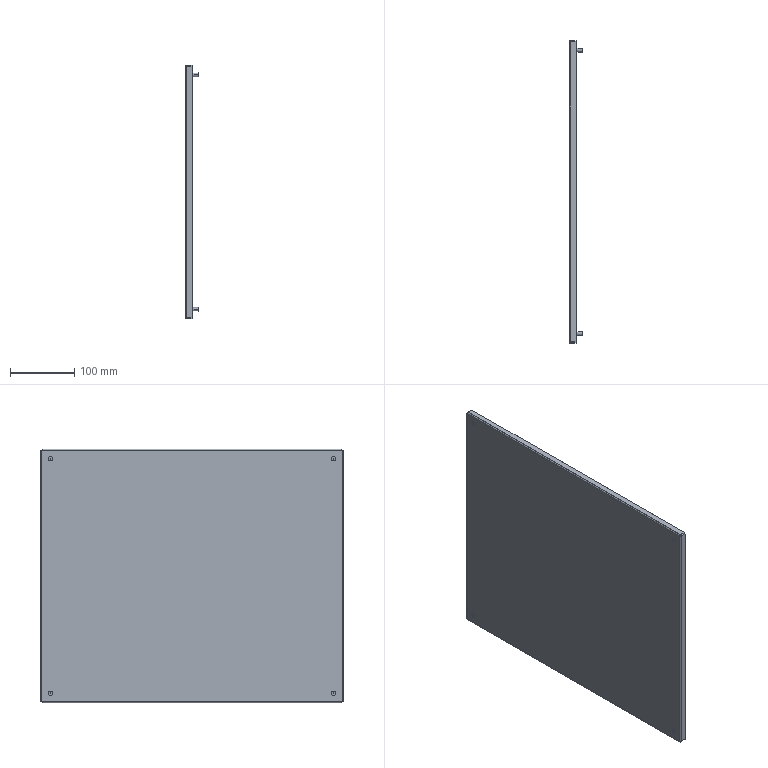Part | SolidWorks | features BaseBody 5 | 5 solids | 66 faces | box 20 x 472 x 396 mm | volume 303544 mm3 | plane 34 | cylinder 32 | commonest cylinder face diameters 1 x8 6 x8 7.2 x8 0.4 x4 3.4 x4